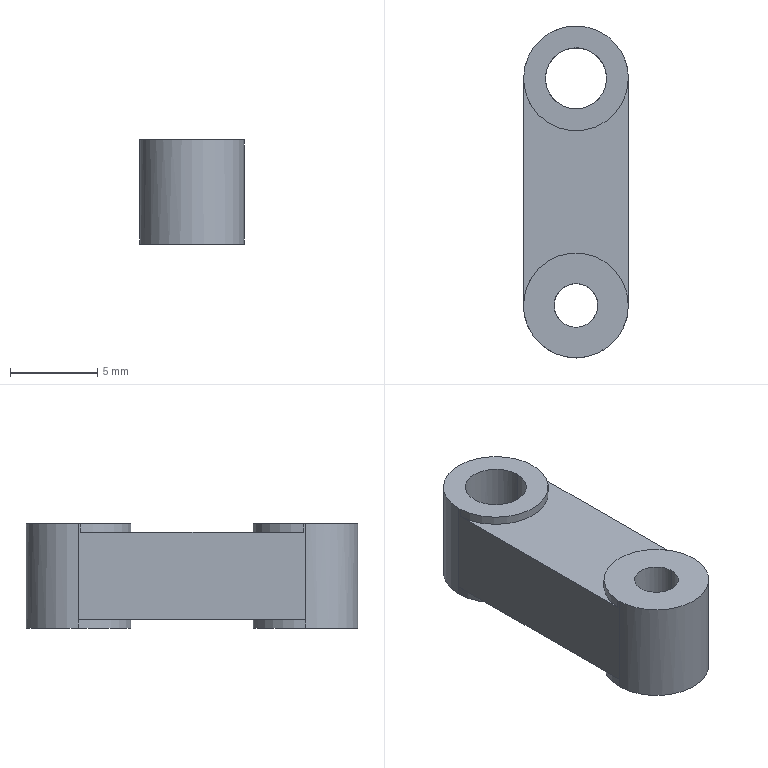Part | SolidWorks | features Cut 3, Extrusion 1, HoleWzd 1 | 1 solid | 20 faces | box 6 x 19 x 6.001 mm | volume 500.74 mm3 | cylinder 10 | plane 10 | commonest cylinder face diameters 6 x6 2.5 x2 3.5 x2
STEP:
#1=CARTESIAN_POINT('',(1.25,-19.,6.001));
#2=VERTEX_POINT('',#1);
#3=CARTESIAN_POINT('',(-1.25,-19.,5.999));
#4=VERTEX_POINT('',#3);
#5=CARTESIAN_POINT('',(1.25,-19.,6.001));
#6=CARTESIAN_POINT('',(1.25,-21.5,6.001));
#7=CARTESIAN_POINT('',(-1.25,-21.5,5.999));
#8=CARTESIAN_POINT('',(-1.25,-19.,5.999));
#9=(BOUNDED_CURVE()B_SPLINE_CURVE(3,(#5,#6,#7,#8),.UNSPECIFIED.,.F.,.F.)B_SPLINE_CURVE_WITH_KNOTS((4,4),(3.142,6.283),.UNSPECIFIED.)CURVE()GEOMETRIC_REPRESENTATION_ITEM()RATIONAL_B_SPLINE_CURVE((1.,0.3333,0.3333,1.))REPRESENTATION_ITEM(''));
#10=EDGE_CURVE('',#2,#4,#9,.T.);
#11=ORIENTED_EDGE('',*,*,#10,.F.);
#12=CARTESIAN_POINT('',(1.25,-19.,0.));
#13=VERTEX_POINT('',#12);
#14=CARTESIAN_POINT('',(1.25,-19.,0.));
#15=DIRECTION('',(0.,0.,-1.));
#16=VECTOR('',#15,1000.);
#17=LINE('',#14,#16);
#18=EDGE_CURVE('',#2,#13,#17,.T.);
#19=ORIENTED_EDGE('',*,*,#18,.T.);
#20=CARTESIAN_POINT('',(-1.25,-19.,0.));
#21=VERTEX_POINT('',#20);
#22=CARTESIAN_POINT('',(0.000000001,-19.,0.));
#23=DIRECTION('',(0.,0.,-1.));
#24=DIRECTION('',(-1.,0.,0.));
#25=AXIS2_PLACEMENT_3D('',#22,#23,#24);
#26=CIRCLE('',#25,1.25);
#27=EDGE_CURVE('',#13,#21,#26,.T.);
#28=ORIENTED_EDGE('',*,*,#27,.T.);
#29=CARTESIAN_POINT('',(-1.25,-19.,0.));
#30=DIRECTION('',(0.,0.,-1.));
#31=VECTOR('',#30,1000.);
#32=LINE('',#29,#31);
#33=EDGE_CURVE('',#4,#21,#32,.T.);
#34=ORIENTED_EDGE('',*,*,#33,.F.);
#35=EDGE_LOOP('',(#11,#19,#28,#34));
#36=FACE_OUTER_BOUND('',#35,.T.);
#37=CARTESIAN_POINT('',(0.000000001,-19.,0.));
#38=DIRECTION('',(0.,0.,-1.));
#39=DIRECTION('',(-1.,0.,0.));
#40=AXIS2_PLACEMENT_3D('',#37,#38,#39);
#41=CYLINDRICAL_SURFACE('',#40,1.25);
#42=ADVANCED_FACE('',(#36),#41,.F.);
#43=CARTESIAN_POINT('',(1.75,-6.,6.001));
#44=VERTEX_POINT('',#43);
#45=CARTESIAN_POINT('',(-1.75,-6.,5.999));
#46=VERTEX_POINT('',#45);
#47=CARTESIAN_POINT('',(1.75,-6.,6.001));
#48=CARTESIAN_POINT('',(1.75,-9.5,6.001));
#49=CARTESIAN_POINT('',(-1.75,-9.5,5.999));
#50=CARTESIAN_POINT('',(-1.75,-6.,5.999));
#51=(BOUNDED_CURVE()B_SPLINE_CURVE(3,(#47,#48,#49,#50),.UNSPECIFIED.,.F.,.F.)B_SPLINE_CURVE_WITH_KNOTS((4,4),(3.142,6.283),.UNSPECIFIED.)CURVE()GEOMETRIC_REPRESENTATION_ITEM()RATIONAL_B_SPLINE_CURVE((1.,0.3333,0.3333,1.))REPRESENTATION_ITEM(''));
#52=EDGE_CURVE('',#44,#46,#51,.T.);
#53=ORIENTED_EDGE('',*,*,#52,.F.);
#54=CARTESIAN_POINT('',(1.75,-6.,0.));
#55=VERTEX_POINT('',#54);
#56=CARTESIAN_POINT('',(1.75,-6.,25.925));
#57=DIRECTION('',(0.,0.,-1.));
#58=VECTOR('',#57,1000.);
#59=LINE('',#56,#58);
#60=EDGE_CURVE('',#44,#55,#59,.T.);
#61=ORIENTED_EDGE('',*,*,#60,.T.);
#62=CARTESIAN_POINT('',(-1.75,-6.,0.));
#63=VERTEX_POINT('',#62);
#64=CARTESIAN_POINT('',(0.,-6.,0.));
#65=DIRECTION('',(0.,0.,1.));
#66=DIRECTION('',(1.,0.,0.));
#67=AXIS2_PLACEMENT_3D('',#64,#65,#66);
#68=CIRCLE('',#67,1.75);
#69=EDGE_CURVE('',#63,#55,#68,.T.);
#70=ORIENTED_EDGE('',*,*,#69,.F.);
#71=CARTESIAN_POINT('',(-1.75,-6.,25.925));
#72=DIRECTION('',(0.,0.,-1.));
#73=VECTOR('',#72,1000.);
#74=LINE('',#71,#73);
#75=EDGE_CURVE('',#46,#63,#74,.T.);
#76=ORIENTED_EDGE('',*,*,#75,.F.);
#77=EDGE_LOOP('',(#53,#61,#70,#76));
#78=FACE_OUTER_BOUND('',#77,.T.);
#79=CARTESIAN_POINT('',(0.,-6.,25.925));
#80=DIRECTION('',(0.,0.,-1.));
#81=DIRECTION('',(-1.,0.,0.));
#82=AXIS2_PLACEMENT_3D('',#79,#80,#81);
#83=CYLINDRICAL_SURFACE('',#82,1.75);
#84=ADVANCED_FACE('',(#78),#83,.F.);
#85=CARTESIAN_POINT('',(3.,-6.,5.501));
#86=VERTEX_POINT('',#85);
#87=CARTESIAN_POINT('',(3.,-6.,0.5));
#88=VERTEX_POINT('',#87);
#89=CARTESIAN_POINT('',(3.,-6.,25.925));
#90=DIRECTION('',(0.,0.,-1.));
#91=VECTOR('',#90,1000.);
#92=LINE('',#89,#91);
#93=EDGE_CURVE('',#86,#88,#92,.T.);
#94=ORIENTED_EDGE('',*,*,#93,.T.);
#95=CARTESIAN_POINT('',(3.,-6.,0.));
#96=VERTEX_POINT('',#95);
#97=CARTESIAN_POINT('',(3.,-6.,25.925));
#98=DIRECTION('',(0.,0.,-1.));
#99=VECTOR('',#98,1000.);
#100=LINE('',#97,#99);
#101=EDGE_CURVE('',#88,#96,#100,.T.);
#102=ORIENTED_EDGE('',*,*,#101,.T.);
#103=CARTESIAN_POINT('',(-3.,-6.,0.));
#104=VERTEX_POINT('',#103);
#105=CARTESIAN_POINT('',(0.,-6.,0.));
#106=DIRECTION('',(0.,0.,1.));
#107=DIRECTION('',(1.,0.,0.));
#108=AXIS2_PLACEMENT_3D('',#105,#106,#107);
#109=CIRCLE('',#108,3.);
#110=EDGE_CURVE('',#96,#104,#109,.T.);
#111=ORIENTED_EDGE('',*,*,#110,.T.);
#112=CARTESIAN_POINT('',(-3.,-6.,0.5));
#113=VERTEX_POINT('',#112);
#114=CARTESIAN_POINT('',(-3.,-6.,25.925));
#115=DIRECTION('',(0.,0.,-1.));
#116=VECTOR('',#115,1000.);
#117=LINE('',#114,#116);
#118=EDGE_CURVE('',#113,#104,#117,.T.);
#119=ORIENTED_EDGE('',*,*,#118,.F.);
#120=CARTESIAN_POINT('',(-3.,-6.,5.999));
#121=VERTEX_POINT('',#120);
#122=CARTESIAN_POINT('',(-3.,-6.,25.925));
#123=DIRECTION('',(0.,0.,-1.));
#124=VECTOR('',#123,1000.);
#125=LINE('',#122,#124);
#126=EDGE_CURVE('',#121,#113,#125,.T.);
#127=ORIENTED_EDGE('',*,*,#126,.F.);
#128=CARTESIAN_POINT('',(3.,-6.,6.001));
#129=VERTEX_POINT('',#128);
#130=CARTESIAN_POINT('',(-3.,-6.,5.999));
#131=CARTESIAN_POINT('',(-3.,-4.243,5.999));
#132=CARTESIAN_POINT('',(-1.757,-3.,5.999));
#133=CARTESIAN_POINT('',(0.,-3.,6.));
#134=CARTESIAN_POINT('',(1.757,-3.,6.001));
#135=CARTESIAN_POINT('',(3.,-4.243,6.001));
#136=CARTESIAN_POINT('',(3.,-6.,6.001));
#137=(BOUNDED_CURVE()B_SPLINE_CURVE(3,(#130,#131,#132,#133,#134,#135,#136),.UNSPECIFIED.,.F.,.F.)B_SPLINE_CURVE_WITH_KNOTS((4,3,4),(0.,1.571,3.142),.UNSPECIFIED.)CURVE()GEOMETRIC_REPRESENTATION_ITEM()RATIONAL_B_SPLINE_CURVE((1.,0.8047,0.8047,1.,0.8047,0.8047,1.))REPRESENTATION_ITEM(''));
#138=EDGE_CURVE('',#121,#129,#137,.T.);
#139=ORIENTED_EDGE('',*,*,#138,.T.);
#140=CARTESIAN_POINT('',(3.,-6.,25.925));
#141=DIRECTION('',(0.,0.,-1.));
#142=VECTOR('',#141,1000.);
#143=LINE('',#140,#142);
#144=EDGE_CURVE('',#129,#86,#143,.T.);
#145=ORIENTED_EDGE('',*,*,#144,.T.);
#146=EDGE_LOOP('',(#94,#102,#111,#119,#127,#139,#145));
#147=FACE_OUTER_BOUND('',#146,.T.);
#148=CARTESIAN_POINT('',(0.,-6.,25.925));
#149=DIRECTION('',(0.,0.,-1.));
#150=DIRECTION('',(-1.,0.,0.));
#151=AXIS2_PLACEMENT_3D('',#148,#149,#150);
#152=CYLINDRICAL_SURFACE('',#151,3.);
#153=ADVANCED_FACE('',(#147),#152,.T.);
#154=CARTESIAN_POINT('',(3.,-19.,0.5));
#155=VERTEX_POINT('',#154);
#156=CARTESIAN_POINT('',(-3.,-19.,0.5));
#157=VERTEX_POINT('',#156);
#158=CARTESIAN_POINT('',(0.000000001,-19.,0.5));
#159=DIRECTION('',(0.,0.,1.));
#160=DIRECTION('',(-1.,0.,0.));
#161=AXIS2_PLACEMENT_3D('',#158,#159,#160);
#162=CIRCLE('',#161,3.);
#163=EDGE_CURVE('',#155,#157,#162,.T.);
#164=ORIENTED_EDGE('',*,*,#163,.F.);
#165=CARTESIAN_POINT('',(3.,-19.,0.));
#166=VERTEX_POINT('',#165);
#167=CARTESIAN_POINT('',(3.,-19.,25.925));
#168=DIRECTION('',(0.,0.,-1.));
#169=VECTOR('',#168,1000.);
#170=LINE('',#167,#169);
#171=EDGE_CURVE('',#155,#166,#170,.T.);
#172=ORIENTED_EDGE('',*,*,#171,.T.);
#173=CARTESIAN_POINT('',(-3.,-19.,0.));
#174=VERTEX_POINT('',#173);
#175=CARTESIAN_POINT('',(0.000000001,-19.,0.));
#176=DIRECTION('',(0.,0.,1.));
#177=DIRECTION('',(1.,0.,0.));
#178=AXIS2_PLACEMENT_3D('',#175,#176,#177);
#179=CIRCLE('',#178,3.);
#180=EDGE_CURVE('',#166,#174,#179,.T.);
#181=ORIENTED_EDGE('',*,*,#180,.T.);
#182=CARTESIAN_POINT('',(-3.,-19.,25.925));
#183=DIRECTION('',(0.,0.,-1.));
#184=VECTOR('',#183,1000.);
#185=LINE('',#182,#184);
#186=EDGE_CURVE('',#157,#174,#185,.T.);
#187=ORIENTED_EDGE('',*,*,#186,.F.);
#188=EDGE_LOOP('',(#164,#172,#181,#187));
#189=FACE_OUTER_BOUND('',#188,.T.);
#190=CARTESIAN_POINT('',(0.000000001,-19.,25.925));
#191=DIRECTION('',(0.,0.,-1.));
#192=DIRECTION('',(-1.,0.,0.));
#193=AXIS2_PLACEMENT_3D('',#190,#191,#192);
#194=CYLINDRICAL_SURFACE('',#193,3.);
#195=ADVANCED_FACE('',(#189),#194,.T.);
#196=CARTESIAN_POINT('',(-1.25,-19.,5.999));
#197=CARTESIAN_POINT('',(-1.25,-16.5,5.999));
#198=CARTESIAN_POINT('',(1.25,-16.5,6.001));
#199=CARTESIAN_POINT('',(1.25,-19.,6.001));
#200=(BOUNDED_CURVE()B_SPLINE_CURVE(3,(#196,#197,#198,#199),.UNSPECIFIED.,.F.,.F.)B_SPLINE_CURVE_WITH_KNOTS((4,4),(0.,3.142),.UNSPECIFIED.)CURVE()GEOMETRIC_REPRESENTATION_ITEM()RATIONAL_B_SPLINE_CURVE((1.,0.3333,0.3333,1.))REPRESENTATION_ITEM(''));
#201=EDGE_CURVE('',#4,#2,#200,.T.);
#202=ORIENTED_EDGE('',*,*,#201,.T.);
#203=ORIENTED_EDGE('',*,*,#10,.T.);
#204=EDGE_LOOP('',(#202,#203));
#205=FACE_BOUND('',#204,.T.);
#206=CARTESIAN_POINT('',(3.,-19.,6.001));
#207=VERTEX_POINT('',#206);
#208=CARTESIAN_POINT('',(-3.,-19.,5.999));
#209=VERTEX_POINT('',#208);
#210=CARTESIAN_POINT('',(3.,-19.,6.001));
#211=CARTESIAN_POINT('',(3.,-25.,6.001));
#212=CARTESIAN_POINT('',(-3.,-25.,5.999));
#213=CARTESIAN_POINT('',(-3.,-19.,5.999));
#214=(BOUNDED_CURVE()B_SPLINE_CURVE(3,(#210,#211,#212,#213),.UNSPECIFIED.,.F.,.F.)B_SPLINE_CURVE_WITH_KNOTS((4,4),(3.142,6.283),.UNSPECIFIED.)CURVE()GEOMETRIC_REPRESENTATION_ITEM()RATIONAL_B_SPLINE_CURVE((1.,0.3333,0.3333,1.))REPRESENTATION_ITEM(''));
#215=EDGE_CURVE('',#207,#209,#214,.T.);
#216=ORIENTED_EDGE('',*,*,#215,.F.);
#217=CARTESIAN_POINT('',(2.997,-19.,6.001));
#218=VERTEX_POINT('',#217);
#219=CARTESIAN_POINT('',(3.497,-19.,6.002));
#220=DIRECTION('',(-1.,0.,-0.0004897));
#221=VECTOR('',#220,1000.);
#222=LINE('',#219,#221);
#223=EDGE_CURVE('',#207,#218,#222,.T.);
#224=ORIENTED_EDGE('',*,*,#223,.T.);
#225=CARTESIAN_POINT('',(-3.,-18.873,5.999));
#226=VERTEX_POINT('',#225);
#227=CARTESIAN_POINT('',(-0.002693,-19.,6.));
#228=DIRECTION('',(-0.0004897,0.,1.));
#229=DIRECTION('',(-1.,0.,-0.0004897));
#230=AXIS2_PLACEMENT_3D('',#227,#228,#229);
#231=CIRCLE('',#230,3.);
#232=EDGE_CURVE('',#218,#226,#231,.T.);
#233=ORIENTED_EDGE('',*,*,#232,.T.);
#234=CARTESIAN_POINT('',(-3.,-19.,5.999));
#235=DIRECTION('',(0.,1.,0.));
#236=VECTOR('',#235,1000.);
#237=LINE('',#234,#236);
#238=EDGE_CURVE('',#209,#226,#237,.T.);
#239=ORIENTED_EDGE('',*,*,#238,.F.);
#240=EDGE_LOOP('',(#216,#224,#233,#239));
#241=FACE_OUTER_BOUND('',#240,.T.);
#242=CARTESIAN_POINT('',(233.645,-29.129,6.114));
#243=DIRECTION('',(0.0004897,0.,-1.));
#244=DIRECTION('',(-1.,0.,-0.0004897));
#245=AXIS2_PLACEMENT_3D('',#242,#243,#244);
#246=PLANE('',#245);
#247=ADVANCED_FACE('',(#205,#241),#246,.F.);
#248=CARTESIAN_POINT('',(-1.75,-6.,5.999));
#249=CARTESIAN_POINT('',(-1.75,-2.5,5.999));
#250=CARTESIAN_POINT('',(1.75,-2.5,6.001));
#251=CARTESIAN_POINT('',(1.75,-6.,6.001));
#252=(BOUNDED_CURVE()B_SPLINE_CURVE(3,(#248,#249,#250,#251),.UNSPECIFIED.,.F.,.F.)B_SPLINE_CURVE_WITH_KNOTS((4,4),(0.,3.142),.UNSPECIFIED.)CURVE()GEOMETRIC_REPRESENTATION_ITEM()RATIONAL_B_SPLINE_CURVE((1.,0.3333,0.3333,1.))REPRESENTATION_ITEM(''));
#253=EDGE_CURVE('',#46,#44,#252,.T.);
#254=ORIENTED_EDGE('',*,*,#253,.T.);
#255=ORIENTED_EDGE('',*,*,#52,.T.);
#256=EDGE_LOOP('',(#254,#255));
#257=FACE_BOUND('',#256,.T.);
#258=CARTESIAN_POINT('',(2.997,-6.,6.001));
#259=VERTEX_POINT('',#258);
#260=CARTESIAN_POINT('',(-3.,-6.127,5.999));
#261=VERTEX_POINT('',#260);
#262=CARTESIAN_POINT('',(-0.002693,-6.,6.));
#263=DIRECTION('',(0.0004897,0.,-1.));
#264=DIRECTION('',(1.,0.,0.0004897));
#265=AXIS2_PLACEMENT_3D('',#262,#263,#264);
#266=CIRCLE('',#265,3.);
#267=EDGE_CURVE('',#259,#261,#266,.T.);
#268=ORIENTED_EDGE('',*,*,#267,.F.);
#269=CARTESIAN_POINT('',(3.497,-6.,6.002));
#270=DIRECTION('',(-1.,0.,-0.0004897));
#271=VECTOR('',#270,1000.);
#272=LINE('',#269,#271);
#273=EDGE_CURVE('',#129,#259,#272,.T.);
#274=ORIENTED_EDGE('',*,*,#273,.F.);
#275=ORIENTED_EDGE('',*,*,#138,.F.);
#276=CARTESIAN_POINT('',(-3.,-19.,5.999));
#277=DIRECTION('',(0.,1.,0.));
#278=VECTOR('',#277,1000.);
#279=LINE('',#276,#278);
#280=EDGE_CURVE('',#261,#121,#279,.T.);
#281=ORIENTED_EDGE('',*,*,#280,.F.);
#282=EDGE_LOOP('',(#268,#274,#275,#281));
#283=FACE_OUTER_BOUND('',#282,.T.);
#284=CARTESIAN_POINT('',(233.645,-29.129,6.114));
#285=DIRECTION('',(0.0004897,0.,-1.));
#286=DIRECTION('',(-1.,0.,-0.0004897));
#287=AXIS2_PLACEMENT_3D('',#284,#285,#286);
#288=PLANE('',#287);
#289=ADVANCED_FACE('',(#257,#283),#288,.F.);
#290=ORIENTED_EDGE('',*,*,#69,.T.);
#291=CARTESIAN_POINT('',(0.,-6.,0.));
#292=DIRECTION('',(0.,0.,1.));
#293=DIRECTION('',(1.,0.,0.));
#294=AXIS2_PLACEMENT_3D('',#291,#292,#293);
#295=CIRCLE('',#294,1.75);
#296=EDGE_CURVE('',#55,#63,#295,.T.);
#297=ORIENTED_EDGE('',*,*,#296,.T.);
#298=EDGE_LOOP('',(#290,#297));
#299=FACE_BOUND('',#298,.T.);
#300=CARTESIAN_POINT('',(0.,-6.,0.));
#301=DIRECTION('',(0.,0.,1.));
#302=DIRECTION('',(1.,0.,0.));
#303=AXIS2_PLACEMENT_3D('',#300,#301,#302);
#304=CIRCLE('',#303,3.);
#305=EDGE_CURVE('',#104,#96,#304,.T.);
#306=ORIENTED_EDGE('',*,*,#305,.F.);
#307=ORIENTED_EDGE('',*,*,#110,.F.);
#308=EDGE_LOOP('',(#306,#307));
#309=FACE_OUTER_BOUND('',#308,.T.);
#310=CARTESIAN_POINT('',(0.000000001,-19.,0.));
#311=DIRECTION('',(0.,0.,1.));
#312=DIRECTION('',(1.,0.,0.));
#313=AXIS2_PLACEMENT_3D('',#310,#311,#312);
#314=PLANE('',#313);
#315=ADVANCED_FACE('',(#299,#309),#314,.F.);
#316=ORIENTED_EDGE('',*,*,#93,.F.);
#317=CARTESIAN_POINT('',(3.,-19.,5.501));
#318=VERTEX_POINT('',#317);
#319=CARTESIAN_POINT('',(3.,-6.,5.501));
#320=DIRECTION('',(0.,-1.,0.));
#321=VECTOR('',#320,1000.);
#322=LINE('',#319,#321);
#323=EDGE_CURVE('',#86,#318,#322,.T.);
#324=ORIENTED_EDGE('',*,*,#323,.T.);
#325=CARTESIAN_POINT('',(3.,-19.,25.925));
#326=DIRECTION('',(0.,0.,-1.));
#327=VECTOR('',#326,1000.);
#328=LINE('',#325,#327);
#329=EDGE_CURVE('',#318,#155,#328,.T.);
#330=ORIENTED_EDGE('',*,*,#329,.T.);
#331=CARTESIAN_POINT('',(3.,-19.,0.5));
#332=DIRECTION('',(0.,-1.,0.));
#333=VECTOR('',#332,1000.);
#334=LINE('',#331,#333);
#335=EDGE_CURVE('',#88,#155,#334,.T.);
#336=ORIENTED_EDGE('',*,*,#335,.F.);
#337=EDGE_LOOP('',(#316,#324,#330,#336));
#338=FACE_OUTER_BOUND('',#337,.T.);
#339=CARTESIAN_POINT('',(3.,-6.,25.925));
#340=DIRECTION('',(-1.,0.,0.));
#341=DIRECTION('',(0.,-1.,0.));
#342=AXIS2_PLACEMENT_3D('',#339,#340,#341);
#343=PLANE('',#342);
#344=ADVANCED_FACE('',(#338),#343,.F.);
#345=CARTESIAN_POINT('',(-3.,-6.121,5.499));
#346=VERTEX_POINT('',#345);
#347=CARTESIAN_POINT('',(-3.,-18.879,5.499));
#348=VERTEX_POINT('',#347);
#349=CARTESIAN_POINT('',(-3.,-19.,5.499));
#350=DIRECTION('',(0.,-1.,0.));
#351=VECTOR('',#350,1000.);
#352=LINE('',#349,#351);
#353=EDGE_CURVE('',#346,#348,#352,.T.);
#354=ORIENTED_EDGE('',*,*,#353,.F.);
#355=CARTESIAN_POINT('',(-3.,-6.121,5.499));
#356=CARTESIAN_POINT('',(-3.,-6.123,5.661));
#357=CARTESIAN_POINT('',(-3.,-6.125,5.828));
#358=CARTESIAN_POINT('',(-3.,-6.127,5.999));
#359=(BOUNDED_CURVE()B_SPLINE_CURVE(3,(#355,#356,#357,#358),.UNSPECIFIED.,.F.,.F.)B_SPLINE_CURVE_WITH_KNOTS((4,4),(3.182,3.184),.UNSPECIFIED.)CURVE()GEOMETRIC_REPRESENTATION_ITEM()RATIONAL_B_SPLINE_CURVE((1.,1.,1.,1.))REPRESENTATION_ITEM(''));
#360=EDGE_CURVE('',#346,#261,#359,.T.);
#361=ORIENTED_EDGE('',*,*,#360,.T.);
#362=ORIENTED_EDGE('',*,*,#280,.T.);
#363=ORIENTED_EDGE('',*,*,#126,.T.);
#364=CARTESIAN_POINT('',(-3.,-6.,0.5));
#365=DIRECTION('',(0.,1.,0.));
#366=VECTOR('',#365,1000.);
#367=LINE('',#364,#366);
#368=EDGE_CURVE('',#157,#113,#367,.T.);
#369=ORIENTED_EDGE('',*,*,#368,.F.);
#370=CARTESIAN_POINT('',(-3.,-19.,25.925));
#371=DIRECTION('',(0.,0.,-1.));
#372=VECTOR('',#371,1000.);
#373=LINE('',#370,#372);
#374=EDGE_CURVE('',#209,#157,#373,.T.);
#375=ORIENTED_EDGE('',*,*,#374,.F.);
#376=ORIENTED_EDGE('',*,*,#238,.T.);
#377=CARTESIAN_POINT('',(-3.,-18.873,5.999));
#378=CARTESIAN_POINT('',(-3.,-18.875,5.828));
#379=CARTESIAN_POINT('',(-3.,-18.877,5.661));
#380=CARTESIAN_POINT('',(-3.,-18.879,5.499));
#381=(BOUNDED_CURVE()B_SPLINE_CURVE(3,(#377,#378,#379,#380),.UNSPECIFIED.,.F.,.F.)B_SPLINE_CURVE_WITH_KNOTS((4,4),(3.099,3.101),.UNSPECIFIED.)CURVE()GEOMETRIC_REPRESENTATION_ITEM()RATIONAL_B_SPLINE_CURVE((1.,1.,1.,1.))REPRESENTATION_ITEM(''));
#382=EDGE_CURVE('',#226,#348,#381,.T.);
#383=ORIENTED_EDGE('',*,*,#382,.T.);
#384=EDGE_LOOP('',(#354,#361,#362,#363,#369,#375,#376,#383));
#385=FACE_OUTER_BOUND('',#384,.T.);
#386=CARTESIAN_POINT('',(-3.,-19.,25.925));
#387=DIRECTION('',(1.,0.,0.));
#388=DIRECTION('',(0.,1.,0.));
#389=AXIS2_PLACEMENT_3D('',#386,#387,#388);
#390=PLANE('',#389);
#391=ADVANCED_FACE('',(#385),#390,.F.);
#392=CARTESIAN_POINT('',(0.000000001,-19.,0.));
#393=DIRECTION('',(0.,0.,-1.));
#394=DIRECTION('',(-1.,0.,0.));
#395=AXIS2_PLACEMENT_3D('',#392,#393,#394);
#396=CIRCLE('',#395,1.25);
#397=EDGE_CURVE('',#21,#13,#396,.T.);
#398=ORIENTED_EDGE('',*,*,#397,.F.);
#399=ORIENTED_EDGE('',*,*,#27,.F.);
#400=EDGE_LOOP('',(#398,#399));
#401=FACE_BOUND('',#400,.T.);
#402=CARTESIAN_POINT('',(0.000000001,-19.,0.));
#403=DIRECTION('',(0.,0.,1.));
#404=DIRECTION('',(1.,0.,0.));
#405=AXIS2_PLACEMENT_3D('',#402,#403,#404);
#406=CIRCLE('',#405,3.);
#407=EDGE_CURVE('',#174,#166,#406,.T.);
#408=ORIENTED_EDGE('',*,*,#407,.F.);
#409=ORIENTED_EDGE('',*,*,#180,.F.);
#410=EDGE_LOOP('',(#408,#409));
#411=FACE_OUTER_BOUND('',#410,.T.);
#412=CARTESIAN_POINT('',(0.000000001,-19.,0.));
#413=DIRECTION('',(0.,0.,1.));
#414=DIRECTION('',(1.,0.,0.));
#415=AXIS2_PLACEMENT_3D('',#412,#413,#414);
#416=PLANE('',#415);
#417=ADVANCED_FACE('',(#401,#411),#416,.F.);
#418=ORIENTED_EDGE('',*,*,#171,.F.);
#419=ORIENTED_EDGE('',*,*,#329,.F.);
#420=CARTESIAN_POINT('',(3.,-19.,25.925));
#421=DIRECTION('',(0.,0.,-1.));
#422=VECTOR('',#421,1000.);
#423=LINE('',#420,#422);
#424=EDGE_CURVE('',#207,#318,#423,.T.);
#425=ORIENTED_EDGE('',*,*,#424,.F.);
#426=ORIENTED_EDGE('',*,*,#215,.T.);
#427=ORIENTED_EDGE('',*,*,#374,.T.);
#428=ORIENTED_EDGE('',*,*,#186,.T.);
#429=ORIENTED_EDGE('',*,*,#407,.T.);
#430=EDGE_LOOP('',(#418,#419,#425,#426,#427,#428,#429));
#431=FACE_OUTER_BOUND('',#430,.T.);
#432=CARTESIAN_POINT('',(0.000000001,-19.,25.925));
#433=DIRECTION('',(0.,0.,-1.));
#434=DIRECTION('',(-1.,0.,0.));
#435=AXIS2_PLACEMENT_3D('',#432,#433,#434);
#436=CYLINDRICAL_SURFACE('',#435,3.);
#437=ADVANCED_FACE('',(#431),#436,.T.);
#438=ORIENTED_EDGE('',*,*,#101,.F.);
#439=CARTESIAN_POINT('',(0.,-6.,0.5));
#440=DIRECTION('',(0.,0.,1.));
#441=DIRECTION('',(-1.,0.,0.));
#442=AXIS2_PLACEMENT_3D('',#439,#440,#441);
#443=CIRCLE('',#442,3.);
#444=EDGE_CURVE('',#113,#88,#443,.T.);
#445=ORIENTED_EDGE('',*,*,#444,.F.);
#446=ORIENTED_EDGE('',*,*,#118,.T.);
#447=ORIENTED_EDGE('',*,*,#305,.T.);
#448=EDGE_LOOP('',(#438,#445,#446,#447));
#449=FACE_OUTER_BOUND('',#448,.T.);
#450=CARTESIAN_POINT('',(0.,-6.,25.925));
#451=DIRECTION('',(0.,0.,-1.));
#452=DIRECTION('',(-1.,0.,0.));
#453=AXIS2_PLACEMENT_3D('',#450,#451,#452);
#454=CYLINDRICAL_SURFACE('',#453,3.);
#455=ADVANCED_FACE('',(#449),#454,.T.);
#456=ORIENTED_EDGE('',*,*,#60,.F.);
#457=ORIENTED_EDGE('',*,*,#253,.F.);
#458=ORIENTED_EDGE('',*,*,#75,.T.);
#459=ORIENTED_EDGE('',*,*,#296,.F.);
#460=EDGE_LOOP('',(#456,#457,#458,#459));
#461=FACE_OUTER_BOUND('',#460,.T.);
#462=CARTESIAN_POINT('',(0.,-6.,25.925));
#463=DIRECTION('',(0.,0.,-1.));
#464=DIRECTION('',(-1.,0.,0.));
#465=AXIS2_PLACEMENT_3D('',#462,#463,#464);
#466=CYLINDRICAL_SURFACE('',#465,1.75);
#467=ADVANCED_FACE('',(#461),#466,.F.);
#468=ORIENTED_EDGE('',*,*,#18,.F.);
#469=ORIENTED_EDGE('',*,*,#201,.F.);
#470=ORIENTED_EDGE('',*,*,#33,.T.);
#471=ORIENTED_EDGE('',*,*,#397,.T.);
#472=EDGE_LOOP('',(#468,#469,#470,#471));
#473=FACE_OUTER_BOUND('',#472,.T.);
#474=CARTESIAN_POINT('',(0.000000001,-19.,0.));
#475=DIRECTION('',(0.,0.,-1.));
#476=DIRECTION('',(-1.,0.,0.));
#477=AXIS2_PLACEMENT_3D('',#474,#475,#476);
#478=CYLINDRICAL_SURFACE('',#477,1.25);
#479=ADVANCED_FACE('',(#473),#478,.F.);
#480=ORIENTED_EDGE('',*,*,#444,.T.);
#481=ORIENTED_EDGE('',*,*,#335,.T.);
#482=ORIENTED_EDGE('',*,*,#163,.T.);
#483=ORIENTED_EDGE('',*,*,#368,.T.);
#484=EDGE_LOOP('',(#480,#481,#482,#483));
#485=FACE_OUTER_BOUND('',#484,.T.);
#486=CARTESIAN_POINT('',(0.,-6.,0.5));
#487=DIRECTION('',(0.,0.,-1.));
#488=DIRECTION('',(-1.,0.,0.));
#489=AXIS2_PLACEMENT_3D('',#486,#487,#488);
#490=PLANE('',#489);
#491=ADVANCED_FACE('',(#485),#490,.T.);
#492=ORIENTED_EDGE('',*,*,#353,.T.);
#493=CARTESIAN_POINT('',(2.998,-19.,5.501));
#494=VERTEX_POINT('',#493);
#495=CARTESIAN_POINT('',(-0.002449,-19.,5.5));
#496=DIRECTION('',(0.0004897,0.,-1.));
#497=DIRECTION('',(1.,0.,0.0004897));
#498=AXIS2_PLACEMENT_3D('',#495,#496,#497);
#499=CIRCLE('',#498,3.);
#500=EDGE_CURVE('',#348,#494,#499,.T.);
#501=ORIENTED_EDGE('',*,*,#500,.T.);
#502=CARTESIAN_POINT('',(3.498,-19.,5.502));
#503=DIRECTION('',(-1.,0.,-0.0004897));
#504=VECTOR('',#503,1000.);
#505=LINE('',#502,#504);
#506=EDGE_CURVE('',#318,#494,#505,.T.);
#507=ORIENTED_EDGE('',*,*,#506,.F.);
#508=ORIENTED_EDGE('',*,*,#323,.F.);
#509=CARTESIAN_POINT('',(2.998,-6.,5.501));
#510=VERTEX_POINT('',#509);
#511=CARTESIAN_POINT('',(3.498,-6.,5.502));
#512=DIRECTION('',(-1.,0.,-0.0004897));
#513=VECTOR('',#512,1000.);
#514=LINE('',#511,#513);
#515=EDGE_CURVE('',#86,#510,#514,.T.);
#516=ORIENTED_EDGE('',*,*,#515,.T.);
#517=CARTESIAN_POINT('',(-0.002449,-6.,5.5));
#518=DIRECTION('',(0.0004897,0.,-1.));
#519=DIRECTION('',(1.,0.,0.0004897));
#520=AXIS2_PLACEMENT_3D('',#517,#518,#519);
#521=CIRCLE('',#520,3.);
#522=EDGE_CURVE('',#510,#346,#521,.T.);
#523=ORIENTED_EDGE('',*,*,#522,.T.);
#524=EDGE_LOOP('',(#492,#501,#507,#508,#516,#523));
#525=FACE_OUTER_BOUND('',#524,.T.);
#526=CARTESIAN_POINT('',(-0.002449,-6.,5.5));
#527=DIRECTION('',(-0.0004897,0.,1.));
#528=DIRECTION('',(1.,0.,0.0004897));
#529=AXIS2_PLACEMENT_3D('',#526,#527,#528);
#530=PLANE('',#529);
#531=ADVANCED_FACE('',(#525),#530,.T.);
#532=ORIENTED_EDGE('',*,*,#522,.F.);
#533=CARTESIAN_POINT('',(2.998,-6.,5.501));
#534=DIRECTION('',(-0.0004897,0.,1.));
#535=VECTOR('',#534,1000.);
#536=LINE('',#533,#535);
#537=EDGE_CURVE('',#510,#259,#536,.T.);
#538=ORIENTED_EDGE('',*,*,#537,.T.);
#539=ORIENTED_EDGE('',*,*,#267,.T.);
#540=ORIENTED_EDGE('',*,*,#360,.F.);
#541=EDGE_LOOP('',(#532,#538,#539,#540));
#542=FACE_OUTER_BOUND('',#541,.T.);
#543=CARTESIAN_POINT('',(-0.002449,-6.,5.5));
#544=DIRECTION('',(-0.0004897,0.,1.));
#545=DIRECTION('',(1.,0.,0.0004897));
#546=AXIS2_PLACEMENT_3D('',#543,#544,#545);
#547=CYLINDRICAL_SURFACE('',#546,3.);
#548=ADVANCED_FACE('',(#542),#547,.T.);
#549=ORIENTED_EDGE('',*,*,#232,.F.);
#550=CARTESIAN_POINT('',(2.998,-19.,5.501));
#551=DIRECTION('',(-0.0004897,0.,1.));
#552=VECTOR('',#551,1000.);
#553=LINE('',#550,#552);
#554=EDGE_CURVE('',#494,#218,#553,.T.);
#555=ORIENTED_EDGE('',*,*,#554,.F.);
#556=ORIENTED_EDGE('',*,*,#500,.F.);
#557=ORIENTED_EDGE('',*,*,#382,.F.);
#558=EDGE_LOOP('',(#549,#555,#556,#557));
#559=FACE_OUTER_BOUND('',#558,.T.);
#560=CARTESIAN_POINT('',(-0.002449,-19.,5.5));
#561=DIRECTION('',(-0.0004897,0.,1.));
#562=DIRECTION('',(1.,0.,0.0004897));
#563=AXIS2_PLACEMENT_3D('',#560,#561,#562);
#564=CYLINDRICAL_SURFACE('',#563,3.);
#565=ADVANCED_FACE('',(#559),#564,.T.);
#566=ORIENTED_EDGE('',*,*,#506,.T.);
#567=ORIENTED_EDGE('',*,*,#554,.T.);
#568=ORIENTED_EDGE('',*,*,#223,.F.);
#569=ORIENTED_EDGE('',*,*,#424,.T.);
#570=EDGE_LOOP('',(#566,#567,#568,#569));
#571=FACE_OUTER_BOUND('',#570,.T.);
#572=CARTESIAN_POINT('',(3.498,-19.,5.502));
#573=DIRECTION('',(0.,-1.,0.));
#574=DIRECTION('',(1.,0.,0.));
#575=AXIS2_PLACEMENT_3D('',#572,#573,#574);
#576=PLANE('',#575);
#577=ADVANCED_FACE('',(#571),#576,.F.);
#578=ORIENTED_EDGE('',*,*,#273,.T.);
#579=ORIENTED_EDGE('',*,*,#537,.F.);
#580=ORIENTED_EDGE('',*,*,#515,.F.);
#581=ORIENTED_EDGE('',*,*,#144,.F.);
#582=EDGE_LOOP('',(#578,#579,#580,#581));
#583=FACE_OUTER_BOUND('',#582,.T.);
#584=CARTESIAN_POINT('',(3.497,-6.,6.002));
#585=DIRECTION('',(0.,1.,0.));
#586=DIRECTION('',(-1.,0.,0.));
#587=AXIS2_PLACEMENT_3D('',#584,#585,#586);
#588=PLANE('',#587);
#589=ADVANCED_FACE('',(#583),#588,.F.);
#590=CLOSED_SHELL('',(#42,#84,#153,#195,#247,#289,#315,#344,#391,#417,#437,#455,#467,#479,#491,#531,#548,#565,#577,#589));
#591=MANIFOLD_SOLID_BREP('',#590);
#592=CARTESIAN_POINT('',(0.,0.,0.));
#593=DIRECTION('',(0.,0.,1.));
#594=DIRECTION('',(1.,0.,0.));
#595=AXIS2_PLACEMENT_3D('',#592,#593,#594);
#596=(LENGTH_UNIT()NAMED_UNIT(*)SI_UNIT(.MILLI.,.METRE.));
#597=UNCERTAINTY_MEASURE_WITH_UNIT(LENGTH_MEASURE(0.00001),#596,'','');
#598=(NAMED_UNIT(*)PLANE_ANGLE_UNIT()SI_UNIT($,.RADIAN.));
#599=(NAMED_UNIT(*)SI_UNIT($,.STERADIAN.)SOLID_ANGLE_UNIT());
#600=(GEOMETRIC_REPRESENTATION_CONTEXT(3)GLOBAL_UNCERTAINTY_ASSIGNED_CONTEXT((#597))GLOBAL_UNIT_ASSIGNED_CONTEXT((#596,#598,#599))REPRESENTATION_CONTEXT('',''));
#601=ADVANCED_BREP_SHAPE_REPRESENTATION('',(#591,#595),#600);